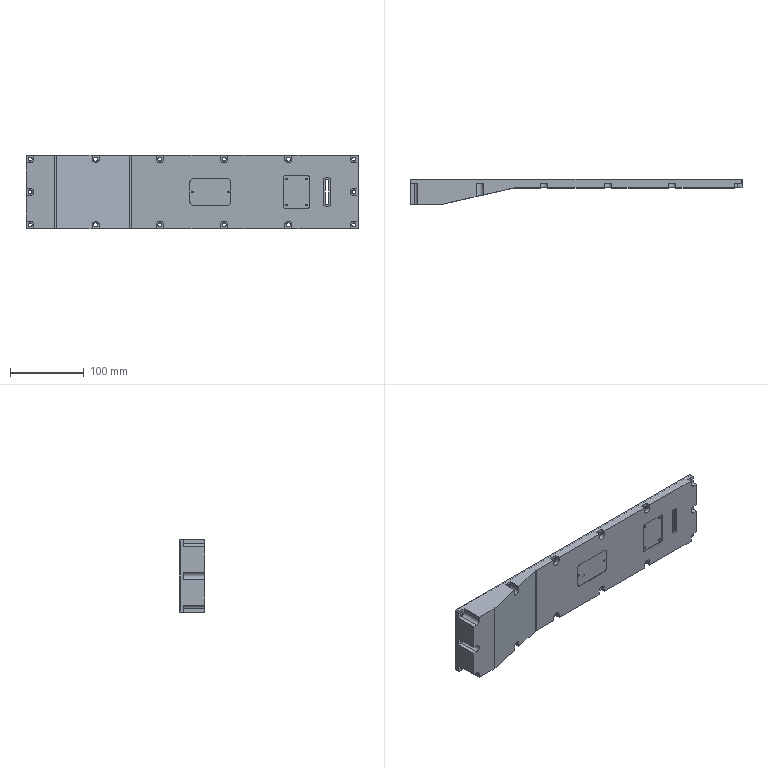Part | 1 solid | 319 faces | box 450 x 35 x 100 mm | volume 257104 mm3 | cylinder 172 | plane 119 | cone 28 | commonest cylinder face diameters 10 x64 2.5 x28 5.5 x28 6 x24 4 x16 8 x8